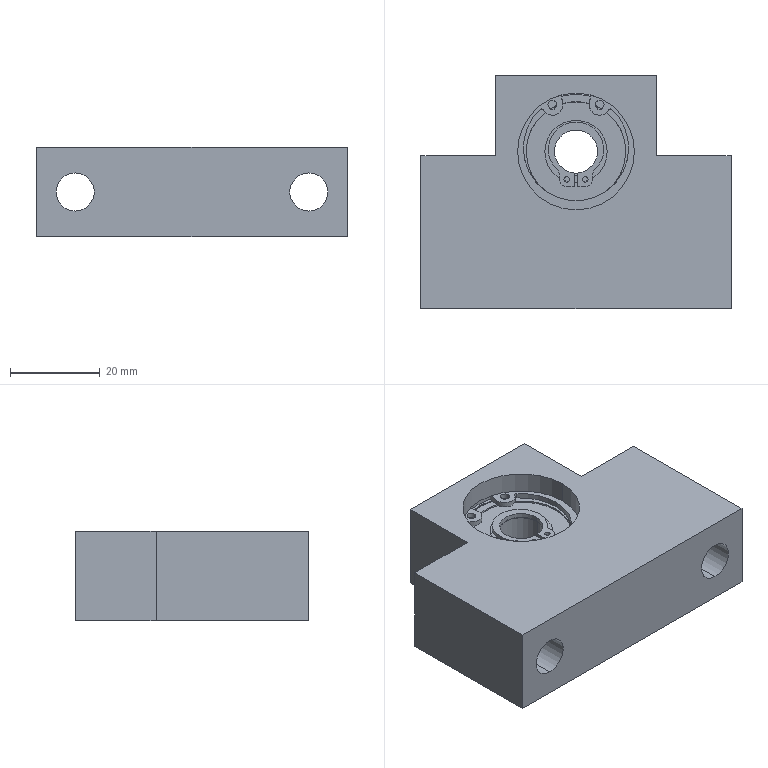Part | STEP file | 001-011-LHF02-R10 | 3 solids | 132 faces | box 69 x 52 x 20 mm | volume 49215 mm3 | cylinder 70 | plane 50 | torus 8 | cone 4 | commonest cylinder face diameters 2 x8 26 x8 4.6 x6 23.472 x6 27.9 x6 1 x4